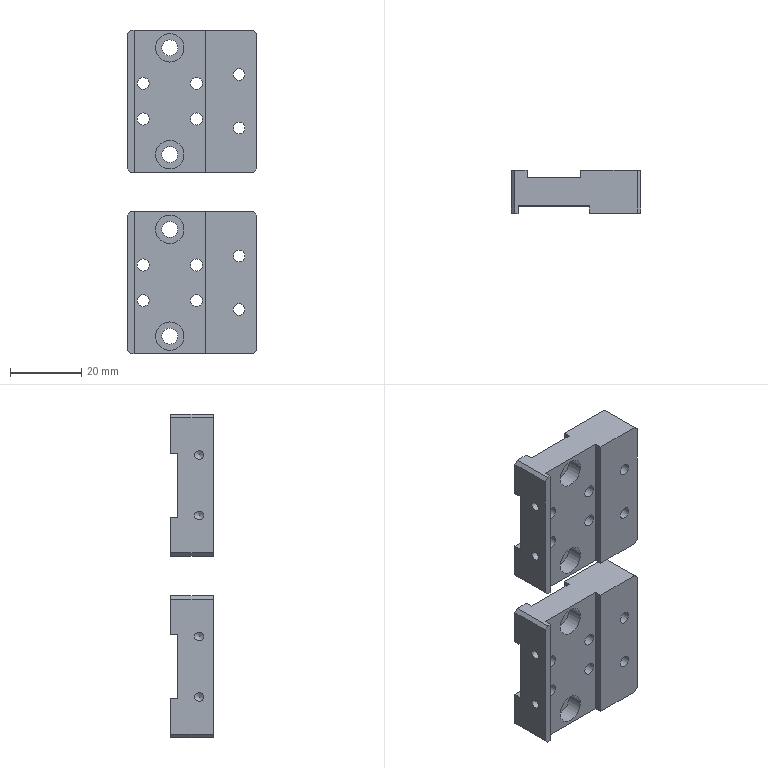CAM job | NX | 3+2 milling, drilling | part box 36.5 x 12 x 91 mm | stock box 41.5 x 15 x 96 mm
Tools:
number,name,description,diameter,corner_radius,flute_length,length,flutes
4,D4,平底铣刀-粗,4.0,0.0,25.0,75.0,2
9,D10,平底铣刀-粗,10.0,0.0,35.0,75.0,2
11,D4-J,平底铣刀-精,4.0,0.0,50.0,75.0,2
7,D6-J,平底铣刀-精,6.0,0.0,25.0,75.0,2
10,D10-J,平底铣刀-精,10.0,0.0,35.0,75.0,2
1,D80R0.8飞刀,圆鼻刀-粗,80.0,0.8,50.0,75.0,2
1,D80R0.8飞刀-J,圆鼻刀-精,80.0,0.8,50.0,75.0,2
2,D6倒角刀,倒角刀,6.0,0.0,3.0,25.0,2
21,M4X0.7,丝锥,3.3,0.0,35.0,50.0,2
13,ZT3.4,钻头,3.4,0.0,35.0,50.0,2
11,ZT4.5,钻头,4.5,0.0,35.0,50.0,2
13,钻头3.3,Twist Drill 3.3 mm,3.3,0.0,35.0,35.008,2
Operations:
program,operation,operation_type,tool,method,geometry_group,spindle_rpm,surface_speed,feed_per_tooth,feed_cut,feed_plunge,cut_length_mm,path_length_mm,cut_time_min,machine_time_min
B,底壁铣飞面一刀开粗_COPY,VolumeBased25DMillingOperation,D80R0.8飞刀,分层开粗-切深K-步距G,W-B,2800.0,703.696,0.5357,3000.0,100.0,1195.164,2274.186,0.3984,0.5063
B,底壁铣飞面一刀精光_COPY,VolumeBased25DMillingOperation,D80R0.8飞刀-J,侧刃精光-切深K-步距G,W-B,4000.0,1005.28,0.125,1000.0,100.0,198.998,234.998,0.199,0.2026
B,底壁铣分层开粗-中_COPY,VolumeBased25DMillingOperation,D10,分层开粗-切深K-步距G,W-B,8000.0,251.32,0.25,4000.0,100.0,1699.802,1734.565,0.425,0.4284
B,铣沉头_1,CylinderMilling,D4,METHOD,W-B,8000.0,100.531,0.1125,1800.0,100.0,724.399,1027.799,0.4024,0.4328
B,铣孔_1,CylinderMilling,D4-J,METHOD,W-B,8000.0,100.531,0.0375,600.0,100.0,70.071,392.271,0.1168,0.149
B,钻倒角_2,Operation,D6倒角刀,METHOD,W-B,8000.0,150.796,0.0625,1000.0,0.0,20.8,157.319,0.0208,0.0345
B,平面去毛刺6X45L_COPY_1,SurfaceContour,D6倒角刀,爬面_倒角-切深0-步距G,W-B,6500.0,122.519,0.1154,1500.0,100.0,612.948,1422.709,0.4086,0.4896
B,底壁铣精光底面-中_COPY,VolumeBased25DMillingOperation,D10-J,精光步距切深关,W-B,8000.0,251.32,0.0625,1000.0,100.0,221.366,247.966,0.2214,0.224
B,底壁铣精光侧面-中-选底面_COPY,VolumeBased25DMillingOperation,D10-J,侧刃精光-切深K-步距G,W-B,8000.0,251.32,0.0625,1000.0,100.0,222.335,249.935,0.2223,0.2251
A,顶面,FaceMilling,D80R0.8飞刀,侧刃精光-切深K-步距G,W-A,4000.0,1005.31,0.125,1000.0,100.0,185.0,221.0,0.185,0.1886
A,外形粗_2,VolumeBased25DMillingOperation,D10,METHOD,W-A,8000.0,251.327,0.3125,5000.0,80.0,9868.893,10021.793,1.974,1.989
A,底壁粗_1,VolumeBased25DMillingOperation,D10,METHOD,W-A,6000.0,113.0,0.2083,3500.0,100.0,1284.169,1469.55,0.3669,0.3854
A,台阶粗_2,CavityMilling,D10,METHOD,W-A,6000.0,188.0,0.25,3500.0,100.0,1280.526,1549.729,0.3659,0.3928
A,打点-深0.8,Operation,D6倒角刀,NONE,W-A,8000.0,150.796,0.0312,500.0,90.0,28.8,318.312,0.0576,0.0866
A,通孔-M4螺纹底孔,Operation,钻头3.3,NONE,W-A,3000.0,31.102,0.05,300.0,90.0,49.966,222.012,0.1666,0.1838
A,沉头孔-钻孔0段,Operation,ZT3.4,NONE,W-A,2800.0,29.908,0.0179,100.0,90.0,96.172,354.622,0.9617,0.9876
A,通孔-5-6,Operation,ZT4.5,NONE,W-A,3000.0,42.411,0.025,150.0,90.0,52.0,232.057,0.3467,0.3647
A,铣孔开粗D4_1,CylinderMilling,D4,NONE,W-A,8000.0,100.531,0.075,1200.0,100.0,954.534,1448.562,0.7954,0.8448
A,铣孔精光D4_1,CylinderMilling,D4-J,精光步距切深关,W-A,8000.0,100.531,0.0312,500.0,100.0,160.587,654.615,0.3212,0.3706
A,清角D4,ZLevelMilling,D4-J,METHOD,W-A,6000.0,75.0,0.1667,2000.0,80.0,1076.122,1298.68,0.5385,0.5607
A,底精_1,VolumeBased25DMillingOperation,D6-J,METHOD,W-A,6000.0,113.0,0.2083,1200.0,100.0,527.848,664.348,0.4399,0.4535
A,底精_2,VolumeBased25DMillingOperation,D6-J,METHOD,W-A,6000.0,113.0,0.2083,1200.0,100.0,199.06,353.56,0.1659,0.1813
A,钻倒角_1,Operation,D6倒角刀,METHOD,W-A,8000.0,150.796,0.0312,500.0,0.0,20.8,170.319,0.0416,0.0566
A,铣倒角_1,PlanarMilling,D6倒角刀,METHOD,W-A,8000.0,150.796,0.0312,500.0,100.0,69.412,330.481,0.1388,0.1649
A,平面去毛刺6X45L_COPY,SurfaceContour,D6倒角刀,爬面_倒角-切深0-步距G,W-A,6500.0,122.519,0.1154,1500.0,100.0,777.763,2445.667,0.5185,0.6853
A,通孔-攻牙M4,Operation,M4X0.7,METHOD,W-A,600.0,6.22,0.0006,0.7,90.0,38.0,198.081,54.286,54.302
A,底侧精_3,VolumeBased25DMillingOperation,D6-J,METHOD,W-A,6000.0,113.0,0.2083,1200.0,100.0,266.554,706.108,0.2221,0.2661
A,底侧精_4,VolumeBased25DMillingOperation,D6-J,METHOD,W-A,6000.0,113.0,0.2083,1200.0,100.0,87.873,225.993,0.0732,0.087
A,外形半精_2,VolumeBased25DMillingOperation,D10-J,METHOD,W-A,8000.0,251.327,0.0625,1000.0,100.0,383.346,446.746,0.3833,0.3897